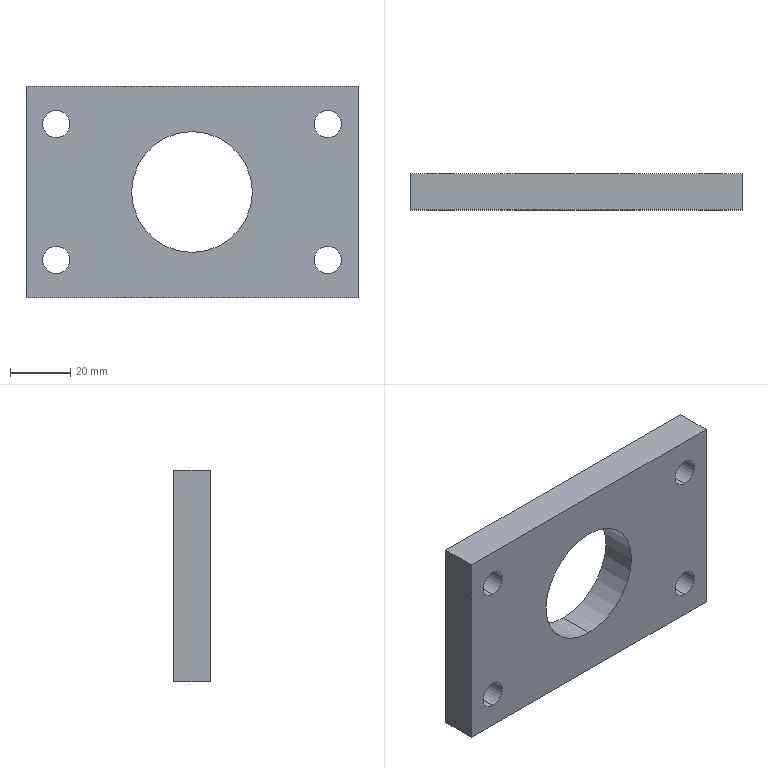Part | SolidWorks | features BaseBody 1 | 1 solid | 16 faces | box 110 x 12 x 70 mm | volume 74267 mm3 | cylinder 10 | plane 6 | commonest cylinder face diameters 9 x8 40 x2
STEP:
#1=CARTESIAN_POINT('',(270.,150.,107.621));
#2=VERTEX_POINT('',#1);
#3=CARTESIAN_POINT('',(270.,150.,116.621));
#4=VERTEX_POINT('',#3);
#5=CARTESIAN_POINT('',(270.,150.,112.121));
#6=DIRECTION('',(0.,1.,0.));
#7=DIRECTION('',(0.,0.,1.));
#8=AXIS2_PLACEMENT_3D('',#5,#6,#7);
#9=CIRCLE('',#8,4.5);
#10=EDGE_CURVE('',#2,#4,#9,.T.);
#11=ORIENTED_EDGE('',*,*,#10,.F.);
#12=CARTESIAN_POINT('',(270.,162.,107.621));
#13=VERTEX_POINT('',#12);
#14=CARTESIAN_POINT('',(270.,162.,107.621));
#15=DIRECTION('',(0.,1.,0.));
#16=VECTOR('',#15,1000.);
#17=LINE('',#14,#16);
#18=EDGE_CURVE('',#2,#13,#17,.T.);
#19=ORIENTED_EDGE('',*,*,#18,.T.);
#20=CARTESIAN_POINT('',(270.,162.,116.621));
#21=VERTEX_POINT('',#20);
#22=CARTESIAN_POINT('',(270.,162.,112.121));
#23=DIRECTION('',(0.,1.,0.));
#24=DIRECTION('',(0.,0.,1.));
#25=AXIS2_PLACEMENT_3D('',#22,#23,#24);
#26=CIRCLE('',#25,4.5);
#27=EDGE_CURVE('',#13,#21,#26,.T.);
#28=ORIENTED_EDGE('',*,*,#27,.T.);
#29=CARTESIAN_POINT('',(270.,162.,116.621));
#30=DIRECTION('',(0.,1.,0.));
#31=VECTOR('',#30,1000.);
#32=LINE('',#29,#31);
#33=EDGE_CURVE('',#4,#21,#32,.T.);
#34=ORIENTED_EDGE('',*,*,#33,.F.);
#35=EDGE_LOOP('',(#11,#19,#28,#34));
#36=FACE_OUTER_BOUND('',#35,.T.);
#37=CARTESIAN_POINT('',(270.,162.,112.121));
#38=DIRECTION('',(0.,1.,0.));
#39=DIRECTION('',(0.,0.,1.));
#40=AXIS2_PLACEMENT_3D('',#37,#38,#39);
#41=CYLINDRICAL_SURFACE('',#40,4.5);
#42=ADVANCED_FACE('',(#36),#41,.F.);
#43=CARTESIAN_POINT('',(270.,150.,152.621));
#44=VERTEX_POINT('',#43);
#45=CARTESIAN_POINT('',(270.,150.,161.621));
#46=VERTEX_POINT('',#45);
#47=CARTESIAN_POINT('',(270.,150.,157.121));
#48=DIRECTION('',(0.,1.,0.));
#49=DIRECTION('',(0.,0.,1.));
#50=AXIS2_PLACEMENT_3D('',#47,#48,#49);
#51=CIRCLE('',#50,4.5);
#52=EDGE_CURVE('',#44,#46,#51,.T.);
#53=ORIENTED_EDGE('',*,*,#52,.F.);
#54=CARTESIAN_POINT('',(270.,162.,152.621));
#55=VERTEX_POINT('',#54);
#56=CARTESIAN_POINT('',(270.,162.,152.621));
#57=DIRECTION('',(0.,1.,0.));
#58=VECTOR('',#57,1000.);
#59=LINE('',#56,#58);
#60=EDGE_CURVE('',#44,#55,#59,.T.);
#61=ORIENTED_EDGE('',*,*,#60,.T.);
#62=CARTESIAN_POINT('',(270.,162.,161.621));
#63=VERTEX_POINT('',#62);
#64=CARTESIAN_POINT('',(270.,162.,157.121));
#65=DIRECTION('',(0.,1.,0.));
#66=DIRECTION('',(0.,0.,1.));
#67=AXIS2_PLACEMENT_3D('',#64,#65,#66);
#68=CIRCLE('',#67,4.5);
#69=EDGE_CURVE('',#55,#63,#68,.T.);
#70=ORIENTED_EDGE('',*,*,#69,.T.);
#71=CARTESIAN_POINT('',(270.,162.,161.621));
#72=DIRECTION('',(0.,1.,0.));
#73=VECTOR('',#72,1000.);
#74=LINE('',#71,#73);
#75=EDGE_CURVE('',#46,#63,#74,.T.);
#76=ORIENTED_EDGE('',*,*,#75,.F.);
#77=EDGE_LOOP('',(#53,#61,#70,#76));
#78=FACE_OUTER_BOUND('',#77,.T.);
#79=CARTESIAN_POINT('',(270.,162.,157.121));
#80=DIRECTION('',(0.,1.,0.));
#81=DIRECTION('',(0.,0.,1.));
#82=AXIS2_PLACEMENT_3D('',#79,#80,#81);
#83=CYLINDRICAL_SURFACE('',#82,4.5);
#84=ADVANCED_FACE('',(#78),#83,.F.);
#85=CARTESIAN_POINT('',(225.,150.,114.621));
#86=VERTEX_POINT('',#85);
#87=CARTESIAN_POINT('',(225.,150.,154.621));
#88=VERTEX_POINT('',#87);
#89=CARTESIAN_POINT('',(225.,150.,134.621));
#90=DIRECTION('',(0.,1.,0.));
#91=DIRECTION('',(0.,0.,1.));
#92=AXIS2_PLACEMENT_3D('',#89,#90,#91);
#93=CIRCLE('',#92,20.);
#94=EDGE_CURVE('',#86,#88,#93,.T.);
#95=ORIENTED_EDGE('',*,*,#94,.F.);
#96=CARTESIAN_POINT('',(225.,162.,114.621));
#97=VERTEX_POINT('',#96);
#98=CARTESIAN_POINT('',(225.,162.,114.621));
#99=DIRECTION('',(0.,1.,0.));
#100=VECTOR('',#99,1000.);
#101=LINE('',#98,#100);
#102=EDGE_CURVE('',#86,#97,#101,.T.);
#103=ORIENTED_EDGE('',*,*,#102,.T.);
#104=CARTESIAN_POINT('',(225.,162.,154.621));
#105=VERTEX_POINT('',#104);
#106=CARTESIAN_POINT('',(225.,162.,134.621));
#107=DIRECTION('',(0.,1.,0.));
#108=DIRECTION('',(0.,0.,1.));
#109=AXIS2_PLACEMENT_3D('',#106,#107,#108);
#110=CIRCLE('',#109,20.);
#111=EDGE_CURVE('',#97,#105,#110,.T.);
#112=ORIENTED_EDGE('',*,*,#111,.T.);
#113=CARTESIAN_POINT('',(225.,162.,154.621));
#114=DIRECTION('',(0.,1.,0.));
#115=VECTOR('',#114,1000.);
#116=LINE('',#113,#115);
#117=EDGE_CURVE('',#88,#105,#116,.T.);
#118=ORIENTED_EDGE('',*,*,#117,.F.);
#119=EDGE_LOOP('',(#95,#103,#112,#118));
#120=FACE_OUTER_BOUND('',#119,.T.);
#121=CARTESIAN_POINT('',(225.,162.,134.621));
#122=DIRECTION('',(0.,1.,0.));
#123=DIRECTION('',(0.,0.,1.));
#124=AXIS2_PLACEMENT_3D('',#121,#122,#123);
#125=CYLINDRICAL_SURFACE('',#124,20.);
#126=ADVANCED_FACE('',(#120),#125,.F.);
#127=CARTESIAN_POINT('',(180.,150.,107.621));
#128=VERTEX_POINT('',#127);
#129=CARTESIAN_POINT('',(180.,150.,116.621));
#130=VERTEX_POINT('',#129);
#131=CARTESIAN_POINT('',(180.,150.,112.121));
#132=DIRECTION('',(0.,1.,0.));
#133=DIRECTION('',(0.,0.,1.));
#134=AXIS2_PLACEMENT_3D('',#131,#132,#133);
#135=CIRCLE('',#134,4.5);
#136=EDGE_CURVE('',#128,#130,#135,.T.);
#137=ORIENTED_EDGE('',*,*,#136,.F.);
#138=CARTESIAN_POINT('',(180.,162.,107.621));
#139=VERTEX_POINT('',#138);
#140=CARTESIAN_POINT('',(180.,162.,107.621));
#141=DIRECTION('',(0.,1.,0.));
#142=VECTOR('',#141,1000.);
#143=LINE('',#140,#142);
#144=EDGE_CURVE('',#128,#139,#143,.T.);
#145=ORIENTED_EDGE('',*,*,#144,.T.);
#146=CARTESIAN_POINT('',(180.,162.,116.621));
#147=VERTEX_POINT('',#146);
#148=CARTESIAN_POINT('',(180.,162.,112.121));
#149=DIRECTION('',(0.,1.,0.));
#150=DIRECTION('',(0.,0.,1.));
#151=AXIS2_PLACEMENT_3D('',#148,#149,#150);
#152=CIRCLE('',#151,4.5);
#153=EDGE_CURVE('',#139,#147,#152,.T.);
#154=ORIENTED_EDGE('',*,*,#153,.T.);
#155=CARTESIAN_POINT('',(180.,162.,116.621));
#156=DIRECTION('',(0.,1.,0.));
#157=VECTOR('',#156,1000.);
#158=LINE('',#155,#157);
#159=EDGE_CURVE('',#130,#147,#158,.T.);
#160=ORIENTED_EDGE('',*,*,#159,.F.);
#161=EDGE_LOOP('',(#137,#145,#154,#160));
#162=FACE_OUTER_BOUND('',#161,.T.);
#163=CARTESIAN_POINT('',(180.,162.,112.121));
#164=DIRECTION('',(0.,1.,0.));
#165=DIRECTION('',(0.,0.,1.));
#166=AXIS2_PLACEMENT_3D('',#163,#164,#165);
#167=CYLINDRICAL_SURFACE('',#166,4.5);
#168=ADVANCED_FACE('',(#162),#167,.F.);
#169=CARTESIAN_POINT('',(180.,150.,152.621));
#170=VERTEX_POINT('',#169);
#171=CARTESIAN_POINT('',(180.,150.,161.621));
#172=VERTEX_POINT('',#171);
#173=CARTESIAN_POINT('',(180.,150.,157.121));
#174=DIRECTION('',(0.,1.,0.));
#175=DIRECTION('',(0.,0.,1.));
#176=AXIS2_PLACEMENT_3D('',#173,#174,#175);
#177=CIRCLE('',#176,4.5);
#178=EDGE_CURVE('',#170,#172,#177,.T.);
#179=ORIENTED_EDGE('',*,*,#178,.F.);
#180=CARTESIAN_POINT('',(180.,162.,152.621));
#181=VERTEX_POINT('',#180);
#182=CARTESIAN_POINT('',(180.,162.,152.621));
#183=DIRECTION('',(0.,1.,0.));
#184=VECTOR('',#183,1000.);
#185=LINE('',#182,#184);
#186=EDGE_CURVE('',#170,#181,#185,.T.);
#187=ORIENTED_EDGE('',*,*,#186,.T.);
#188=CARTESIAN_POINT('',(180.,162.,161.621));
#189=VERTEX_POINT('',#188);
#190=CARTESIAN_POINT('',(180.,162.,157.121));
#191=DIRECTION('',(0.,1.,0.));
#192=DIRECTION('',(0.,0.,1.));
#193=AXIS2_PLACEMENT_3D('',#190,#191,#192);
#194=CIRCLE('',#193,4.5);
#195=EDGE_CURVE('',#181,#189,#194,.T.);
#196=ORIENTED_EDGE('',*,*,#195,.T.);
#197=CARTESIAN_POINT('',(180.,162.,161.621));
#198=DIRECTION('',(0.,1.,0.));
#199=VECTOR('',#198,1000.);
#200=LINE('',#197,#199);
#201=EDGE_CURVE('',#172,#189,#200,.T.);
#202=ORIENTED_EDGE('',*,*,#201,.F.);
#203=EDGE_LOOP('',(#179,#187,#196,#202));
#204=FACE_OUTER_BOUND('',#203,.T.);
#205=CARTESIAN_POINT('',(180.,162.,157.121));
#206=DIRECTION('',(0.,1.,0.));
#207=DIRECTION('',(0.,0.,1.));
#208=AXIS2_PLACEMENT_3D('',#205,#206,#207);
#209=CYLINDRICAL_SURFACE('',#208,4.5);
#210=ADVANCED_FACE('',(#204),#209,.F.);
#211=CARTESIAN_POINT('',(280.,162.,169.621));
#212=VERTEX_POINT('',#211);
#213=CARTESIAN_POINT('',(170.,162.,169.621));
#214=VERTEX_POINT('',#213);
#215=CARTESIAN_POINT('',(225.,162.,169.621));
#216=DIRECTION('',(-1.,0.,0.));
#217=VECTOR('',#216,1000.);
#218=LINE('',#215,#217);
#219=EDGE_CURVE('',#212,#214,#218,.T.);
#220=ORIENTED_EDGE('',*,*,#219,.F.);
#221=CARTESIAN_POINT('',(280.,162.,99.621));
#222=VERTEX_POINT('',#221);
#223=CARTESIAN_POINT('',(280.,162.,134.621));
#224=DIRECTION('',(0.,0.,1.));
#225=VECTOR('',#224,1000.);
#226=LINE('',#223,#225);
#227=EDGE_CURVE('',#222,#212,#226,.T.);
#228=ORIENTED_EDGE('',*,*,#227,.F.);
#229=CARTESIAN_POINT('',(170.,162.,99.621));
#230=VERTEX_POINT('',#229);
#231=CARTESIAN_POINT('',(225.,162.,99.621));
#232=DIRECTION('',(1.,0.,0.));
#233=VECTOR('',#232,1000.);
#234=LINE('',#231,#233);
#235=EDGE_CURVE('',#230,#222,#234,.T.);
#236=ORIENTED_EDGE('',*,*,#235,.F.);
#237=CARTESIAN_POINT('',(170.,162.,134.621));
#238=DIRECTION('',(0.,0.,-1.));
#239=VECTOR('',#238,1000.);
#240=LINE('',#237,#239);
#241=EDGE_CURVE('',#214,#230,#240,.T.);
#242=ORIENTED_EDGE('',*,*,#241,.F.);
#243=EDGE_LOOP('',(#220,#228,#236,#242));
#244=FACE_OUTER_BOUND('',#243,.T.);
#245=CARTESIAN_POINT('',(270.,162.,112.121));
#246=DIRECTION('',(0.,1.,0.));
#247=DIRECTION('',(0.,0.,1.));
#248=AXIS2_PLACEMENT_3D('',#245,#246,#247);
#249=CIRCLE('',#248,4.5);
#250=EDGE_CURVE('',#21,#13,#249,.T.);
#251=ORIENTED_EDGE('',*,*,#250,.F.);
#252=ORIENTED_EDGE('',*,*,#27,.F.);
#253=EDGE_LOOP('',(#251,#252));
#254=FACE_BOUND('',#253,.T.);
#255=CARTESIAN_POINT('',(270.,162.,157.121));
#256=DIRECTION('',(0.,1.,0.));
#257=DIRECTION('',(0.,0.,1.));
#258=AXIS2_PLACEMENT_3D('',#255,#256,#257);
#259=CIRCLE('',#258,4.5);
#260=EDGE_CURVE('',#63,#55,#259,.T.);
#261=ORIENTED_EDGE('',*,*,#260,.F.);
#262=ORIENTED_EDGE('',*,*,#69,.F.);
#263=EDGE_LOOP('',(#261,#262));
#264=FACE_BOUND('',#263,.T.);
#265=CARTESIAN_POINT('',(225.,162.,134.621));
#266=DIRECTION('',(0.,1.,0.));
#267=DIRECTION('',(0.,0.,1.));
#268=AXIS2_PLACEMENT_3D('',#265,#266,#267);
#269=CIRCLE('',#268,20.);
#270=EDGE_CURVE('',#105,#97,#269,.T.);
#271=ORIENTED_EDGE('',*,*,#270,.F.);
#272=ORIENTED_EDGE('',*,*,#111,.F.);
#273=EDGE_LOOP('',(#271,#272));
#274=FACE_BOUND('',#273,.T.);
#275=CARTESIAN_POINT('',(180.,162.,112.121));
#276=DIRECTION('',(0.,1.,0.));
#277=DIRECTION('',(0.,0.,1.));
#278=AXIS2_PLACEMENT_3D('',#275,#276,#277);
#279=CIRCLE('',#278,4.5);
#280=EDGE_CURVE('',#147,#139,#279,.T.);
#281=ORIENTED_EDGE('',*,*,#280,.F.);
#282=ORIENTED_EDGE('',*,*,#153,.F.);
#283=EDGE_LOOP('',(#281,#282));
#284=FACE_BOUND('',#283,.T.);
#285=CARTESIAN_POINT('',(180.,162.,157.121));
#286=DIRECTION('',(0.,1.,0.));
#287=DIRECTION('',(0.,0.,1.));
#288=AXIS2_PLACEMENT_3D('',#285,#286,#287);
#289=CIRCLE('',#288,4.5);
#290=EDGE_CURVE('',#189,#181,#289,.T.);
#291=ORIENTED_EDGE('',*,*,#290,.F.);
#292=ORIENTED_EDGE('',*,*,#195,.F.);
#293=EDGE_LOOP('',(#291,#292));
#294=FACE_BOUND('',#293,.T.);
#295=CARTESIAN_POINT('',(225.,162.,134.621));
#296=DIRECTION('',(0.,-1.,0.));
#297=DIRECTION('',(0.,0.,-1.));
#298=AXIS2_PLACEMENT_3D('',#295,#296,#297);
#299=PLANE('',#298);
#300=ADVANCED_FACE('',(#244,#254,#264,#274,#284,#294),#299,.F.);
#301=CARTESIAN_POINT('',(170.,150.,99.621));
#302=VERTEX_POINT('',#301);
#303=CARTESIAN_POINT('',(170.,150.,169.621));
#304=VERTEX_POINT('',#303);
#305=CARTESIAN_POINT('',(170.,150.,108.621));
#306=DIRECTION('',(0.,0.,1.));
#307=VECTOR('',#306,1000.);
#308=LINE('',#305,#307);
#309=EDGE_CURVE('',#302,#304,#308,.T.);
#310=ORIENTED_EDGE('',*,*,#309,.T.);
#311=CARTESIAN_POINT('',(170.,162.,169.621));
#312=DIRECTION('',(0.,1.,0.));
#313=VECTOR('',#312,1000.);
#314=LINE('',#311,#313);
#315=EDGE_CURVE('',#304,#214,#314,.T.);
#316=ORIENTED_EDGE('',*,*,#315,.T.);
#317=ORIENTED_EDGE('',*,*,#241,.T.);
#318=CARTESIAN_POINT('',(170.,162.,99.621));
#319=DIRECTION('',(0.,-1.,0.));
#320=VECTOR('',#319,1000.);
#321=LINE('',#318,#320);
#322=EDGE_CURVE('',#230,#302,#321,.T.);
#323=ORIENTED_EDGE('',*,*,#322,.T.);
#324=EDGE_LOOP('',(#310,#316,#317,#323));
#325=FACE_OUTER_BOUND('',#324,.T.);
#326=CARTESIAN_POINT('',(170.,162.,108.621));
#327=DIRECTION('',(-1.,0.,0.));
#328=DIRECTION('',(0.,0.,1.));
#329=AXIS2_PLACEMENT_3D('',#326,#327,#328);
#330=PLANE('',#329);
#331=ADVANCED_FACE('',(#325),#330,.T.);
#332=CARTESIAN_POINT('',(280.,150.,169.621));
#333=VERTEX_POINT('',#332);
#334=CARTESIAN_POINT('',(179.,150.,169.621));
#335=DIRECTION('',(1.,0.,0.));
#336=VECTOR('',#335,1000.);
#337=LINE('',#334,#336);
#338=EDGE_CURVE('',#304,#333,#337,.T.);
#339=ORIENTED_EDGE('',*,*,#338,.T.);
#340=CARTESIAN_POINT('',(280.,162.,169.621));
#341=DIRECTION('',(0.,1.,0.));
#342=VECTOR('',#341,1000.);
#343=LINE('',#340,#342);
#344=EDGE_CURVE('',#333,#212,#343,.T.);
#345=ORIENTED_EDGE('',*,*,#344,.T.);
#346=ORIENTED_EDGE('',*,*,#219,.T.);
#347=ORIENTED_EDGE('',*,*,#315,.F.);
#348=EDGE_LOOP('',(#339,#345,#346,#347));
#349=FACE_OUTER_BOUND('',#348,.T.);
#350=CARTESIAN_POINT('',(179.,162.,169.621));
#351=DIRECTION('',(0.,0.,1.));
#352=DIRECTION('',(1.,0.,0.));
#353=AXIS2_PLACEMENT_3D('',#350,#351,#352);
#354=PLANE('',#353);
#355=ADVANCED_FACE('',(#349),#354,.T.);
#356=CARTESIAN_POINT('',(280.,150.,99.621));
#357=VERTEX_POINT('',#356);
#358=CARTESIAN_POINT('',(280.,150.,160.621));
#359=DIRECTION('',(0.,0.,-1.));
#360=VECTOR('',#359,1000.);
#361=LINE('',#358,#360);
#362=EDGE_CURVE('',#333,#357,#361,.T.);
#363=ORIENTED_EDGE('',*,*,#362,.T.);
#364=CARTESIAN_POINT('',(280.,162.,99.621));
#365=DIRECTION('',(0.,1.,0.));
#366=VECTOR('',#365,1000.);
#367=LINE('',#364,#366);
#368=EDGE_CURVE('',#357,#222,#367,.T.);
#369=ORIENTED_EDGE('',*,*,#368,.T.);
#370=ORIENTED_EDGE('',*,*,#227,.T.);
#371=ORIENTED_EDGE('',*,*,#344,.F.);
#372=EDGE_LOOP('',(#363,#369,#370,#371));
#373=FACE_OUTER_BOUND('',#372,.T.);
#374=CARTESIAN_POINT('',(280.,162.,160.621));
#375=DIRECTION('',(1.,0.,0.));
#376=DIRECTION('',(0.,0.,-1.));
#377=AXIS2_PLACEMENT_3D('',#374,#375,#376);
#378=PLANE('',#377);
#379=ADVANCED_FACE('',(#373),#378,.T.);
#380=CARTESIAN_POINT('',(271.,150.,99.621));
#381=DIRECTION('',(-1.,0.,0.));
#382=VECTOR('',#381,1000.);
#383=LINE('',#380,#382);
#384=EDGE_CURVE('',#357,#302,#383,.T.);
#385=ORIENTED_EDGE('',*,*,#384,.T.);
#386=ORIENTED_EDGE('',*,*,#322,.F.);
#387=ORIENTED_EDGE('',*,*,#235,.T.);
#388=ORIENTED_EDGE('',*,*,#368,.F.);
#389=EDGE_LOOP('',(#385,#386,#387,#388));
#390=FACE_OUTER_BOUND('',#389,.T.);
#391=CARTESIAN_POINT('',(271.,162.,99.621));
#392=DIRECTION('',(0.,0.,-1.));
#393=DIRECTION('',(-1.,0.,0.));
#394=AXIS2_PLACEMENT_3D('',#391,#392,#393);
#395=PLANE('',#394);
#396=ADVANCED_FACE('',(#390),#395,.T.);
#397=ORIENTED_EDGE('',*,*,#18,.F.);
#398=CARTESIAN_POINT('',(270.,150.,112.121));
#399=DIRECTION('',(0.,1.,0.));
#400=DIRECTION('',(0.,0.,1.));
#401=AXIS2_PLACEMENT_3D('',#398,#399,#400);
#402=CIRCLE('',#401,4.5);
#403=EDGE_CURVE('',#4,#2,#402,.T.);
#404=ORIENTED_EDGE('',*,*,#403,.F.);
#405=ORIENTED_EDGE('',*,*,#33,.T.);
#406=ORIENTED_EDGE('',*,*,#250,.T.);
#407=EDGE_LOOP('',(#397,#404,#405,#406));
#408=FACE_OUTER_BOUND('',#407,.T.);
#409=CARTESIAN_POINT('',(270.,162.,112.121));
#410=DIRECTION('',(0.,1.,0.));
#411=DIRECTION('',(0.,0.,1.));
#412=AXIS2_PLACEMENT_3D('',#409,#410,#411);
#413=CYLINDRICAL_SURFACE('',#412,4.5);
#414=ADVANCED_FACE('',(#408),#413,.F.);
#415=ORIENTED_EDGE('',*,*,#60,.F.);
#416=CARTESIAN_POINT('',(270.,150.,157.121));
#417=DIRECTION('',(0.,1.,0.));
#418=DIRECTION('',(0.,0.,1.));
#419=AXIS2_PLACEMENT_3D('',#416,#417,#418);
#420=CIRCLE('',#419,4.5);
#421=EDGE_CURVE('',#46,#44,#420,.T.);
#422=ORIENTED_EDGE('',*,*,#421,.F.);
#423=ORIENTED_EDGE('',*,*,#75,.T.);
#424=ORIENTED_EDGE('',*,*,#260,.T.);
#425=EDGE_LOOP('',(#415,#422,#423,#424));
#426=FACE_OUTER_BOUND('',#425,.T.);
#427=CARTESIAN_POINT('',(270.,162.,157.121));
#428=DIRECTION('',(0.,1.,0.));
#429=DIRECTION('',(0.,0.,1.));
#430=AXIS2_PLACEMENT_3D('',#427,#428,#429);
#431=CYLINDRICAL_SURFACE('',#430,4.5);
#432=ADVANCED_FACE('',(#426),#431,.F.);
#433=ORIENTED_EDGE('',*,*,#102,.F.);
#434=CARTESIAN_POINT('',(225.,150.,134.621));
#435=DIRECTION('',(0.,1.,0.));
#436=DIRECTION('',(0.,0.,1.));
#437=AXIS2_PLACEMENT_3D('',#434,#435,#436);
#438=CIRCLE('',#437,20.);
#439=EDGE_CURVE('',#88,#86,#438,.T.);
#440=ORIENTED_EDGE('',*,*,#439,.F.);
#441=ORIENTED_EDGE('',*,*,#117,.T.);
#442=ORIENTED_EDGE('',*,*,#270,.T.);
#443=EDGE_LOOP('',(#433,#440,#441,#442));
#444=FACE_OUTER_BOUND('',#443,.T.);
#445=CARTESIAN_POINT('',(225.,162.,134.621));
#446=DIRECTION('',(0.,1.,0.));
#447=DIRECTION('',(0.,0.,1.));
#448=AXIS2_PLACEMENT_3D('',#445,#446,#447);
#449=CYLINDRICAL_SURFACE('',#448,20.);
#450=ADVANCED_FACE('',(#444),#449,.F.);
#451=ORIENTED_EDGE('',*,*,#144,.F.);
#452=CARTESIAN_POINT('',(180.,150.,112.121));
#453=DIRECTION('',(0.,1.,0.));
#454=DIRECTION('',(0.,0.,1.));
#455=AXIS2_PLACEMENT_3D('',#452,#453,#454);
#456=CIRCLE('',#455,4.5);
#457=EDGE_CURVE('',#130,#128,#456,.T.);
#458=ORIENTED_EDGE('',*,*,#457,.F.);
#459=ORIENTED_EDGE('',*,*,#159,.T.);
#460=ORIENTED_EDGE('',*,*,#280,.T.);
#461=EDGE_LOOP('',(#451,#458,#459,#460));
#462=FACE_OUTER_BOUND('',#461,.T.);
#463=CARTESIAN_POINT('',(180.,162.,112.121));
#464=DIRECTION('',(0.,1.,0.));
#465=DIRECTION('',(0.,0.,1.));
#466=AXIS2_PLACEMENT_3D('',#463,#464,#465);
#467=CYLINDRICAL_SURFACE('',#466,4.5);
#468=ADVANCED_FACE('',(#462),#467,.F.);
#469=ORIENTED_EDGE('',*,*,#186,.F.);
#470=CARTESIAN_POINT('',(180.,150.,157.121));
#471=DIRECTION('',(0.,1.,0.));
#472=DIRECTION('',(0.,0.,1.));
#473=AXIS2_PLACEMENT_3D('',#470,#471,#472);
#474=CIRCLE('',#473,4.5);
#475=EDGE_CURVE('',#172,#170,#474,.T.);
#476=ORIENTED_EDGE('',*,*,#475,.F.);
#477=ORIENTED_EDGE('',*,*,#201,.T.);
#478=ORIENTED_EDGE('',*,*,#290,.T.);
#479=EDGE_LOOP('',(#469,#476,#477,#478));
#480=FACE_OUTER_BOUND('',#479,.T.);
#481=CARTESIAN_POINT('',(180.,162.,157.121));
#482=DIRECTION('',(0.,1.,0.));
#483=DIRECTION('',(0.,0.,1.));
#484=AXIS2_PLACEMENT_3D('',#481,#482,#483);
#485=CYLINDRICAL_SURFACE('',#484,4.5);
#486=ADVANCED_FACE('',(#480),#485,.F.);
#487=ORIENTED_EDGE('',*,*,#384,.F.);
#488=ORIENTED_EDGE('',*,*,#362,.F.);
#489=ORIENTED_EDGE('',*,*,#338,.F.);
#490=ORIENTED_EDGE('',*,*,#309,.F.);
#491=EDGE_LOOP('',(#487,#488,#489,#490));
#492=FACE_OUTER_BOUND('',#491,.T.);
#493=ORIENTED_EDGE('',*,*,#403,.T.);
#494=ORIENTED_EDGE('',*,*,#10,.T.);
#495=EDGE_LOOP('',(#493,#494));
#496=FACE_BOUND('',#495,.T.);
#497=ORIENTED_EDGE('',*,*,#421,.T.);
#498=ORIENTED_EDGE('',*,*,#52,.T.);
#499=EDGE_LOOP('',(#497,#498));
#500=FACE_BOUND('',#499,.T.);
#501=ORIENTED_EDGE('',*,*,#439,.T.);
#502=ORIENTED_EDGE('',*,*,#94,.T.);
#503=EDGE_LOOP('',(#501,#502));
#504=FACE_BOUND('',#503,.T.);
#505=ORIENTED_EDGE('',*,*,#457,.T.);
#506=ORIENTED_EDGE('',*,*,#136,.T.);
#507=EDGE_LOOP('',(#505,#506));
#508=FACE_BOUND('',#507,.T.);
#509=ORIENTED_EDGE('',*,*,#475,.T.);
#510=ORIENTED_EDGE('',*,*,#178,.T.);
#511=EDGE_LOOP('',(#509,#510));
#512=FACE_BOUND('',#511,.T.);
#513=CARTESIAN_POINT('',(225.,150.,134.621));
#514=DIRECTION('',(0.,-1.,0.));
#515=DIRECTION('',(0.,0.,-1.));
#516=AXIS2_PLACEMENT_3D('',#513,#514,#515);
#517=PLANE('',#516);
#518=ADVANCED_FACE('',(#492,#496,#500,#504,#508,#512),#517,.T.);
#519=CLOSED_SHELL('',(#42,#84,#126,#168,#210,#300,#331,#355,#379,#396,#414,#432,#450,#468,#486,#518));
#520=MANIFOLD_SOLID_BREP('',#519);
#521=CARTESIAN_POINT('',(0.,0.,0.));
#522=DIRECTION('',(0.,0.,1.));
#523=DIRECTION('',(1.,0.,0.));
#524=AXIS2_PLACEMENT_3D('',#521,#522,#523);
#525=(LENGTH_UNIT()NAMED_UNIT(*)SI_UNIT(.MILLI.,.METRE.));
#526=UNCERTAINTY_MEASURE_WITH_UNIT(LENGTH_MEASURE(0.00001),#525,'','');
#527=(NAMED_UNIT(*)PLANE_ANGLE_UNIT()SI_UNIT($,.RADIAN.));
#528=(NAMED_UNIT(*)SI_UNIT($,.STERADIAN.)SOLID_ANGLE_UNIT());
#529=(GEOMETRIC_REPRESENTATION_CONTEXT(3)GLOBAL_UNCERTAINTY_ASSIGNED_CONTEXT((#526))GLOBAL_UNIT_ASSIGNED_CONTEXT((#525,#527,#528))REPRESENTATION_CONTEXT('',''));
#530=ADVANCED_BREP_SHAPE_REPRESENTATION('',(#520,#524),#529);